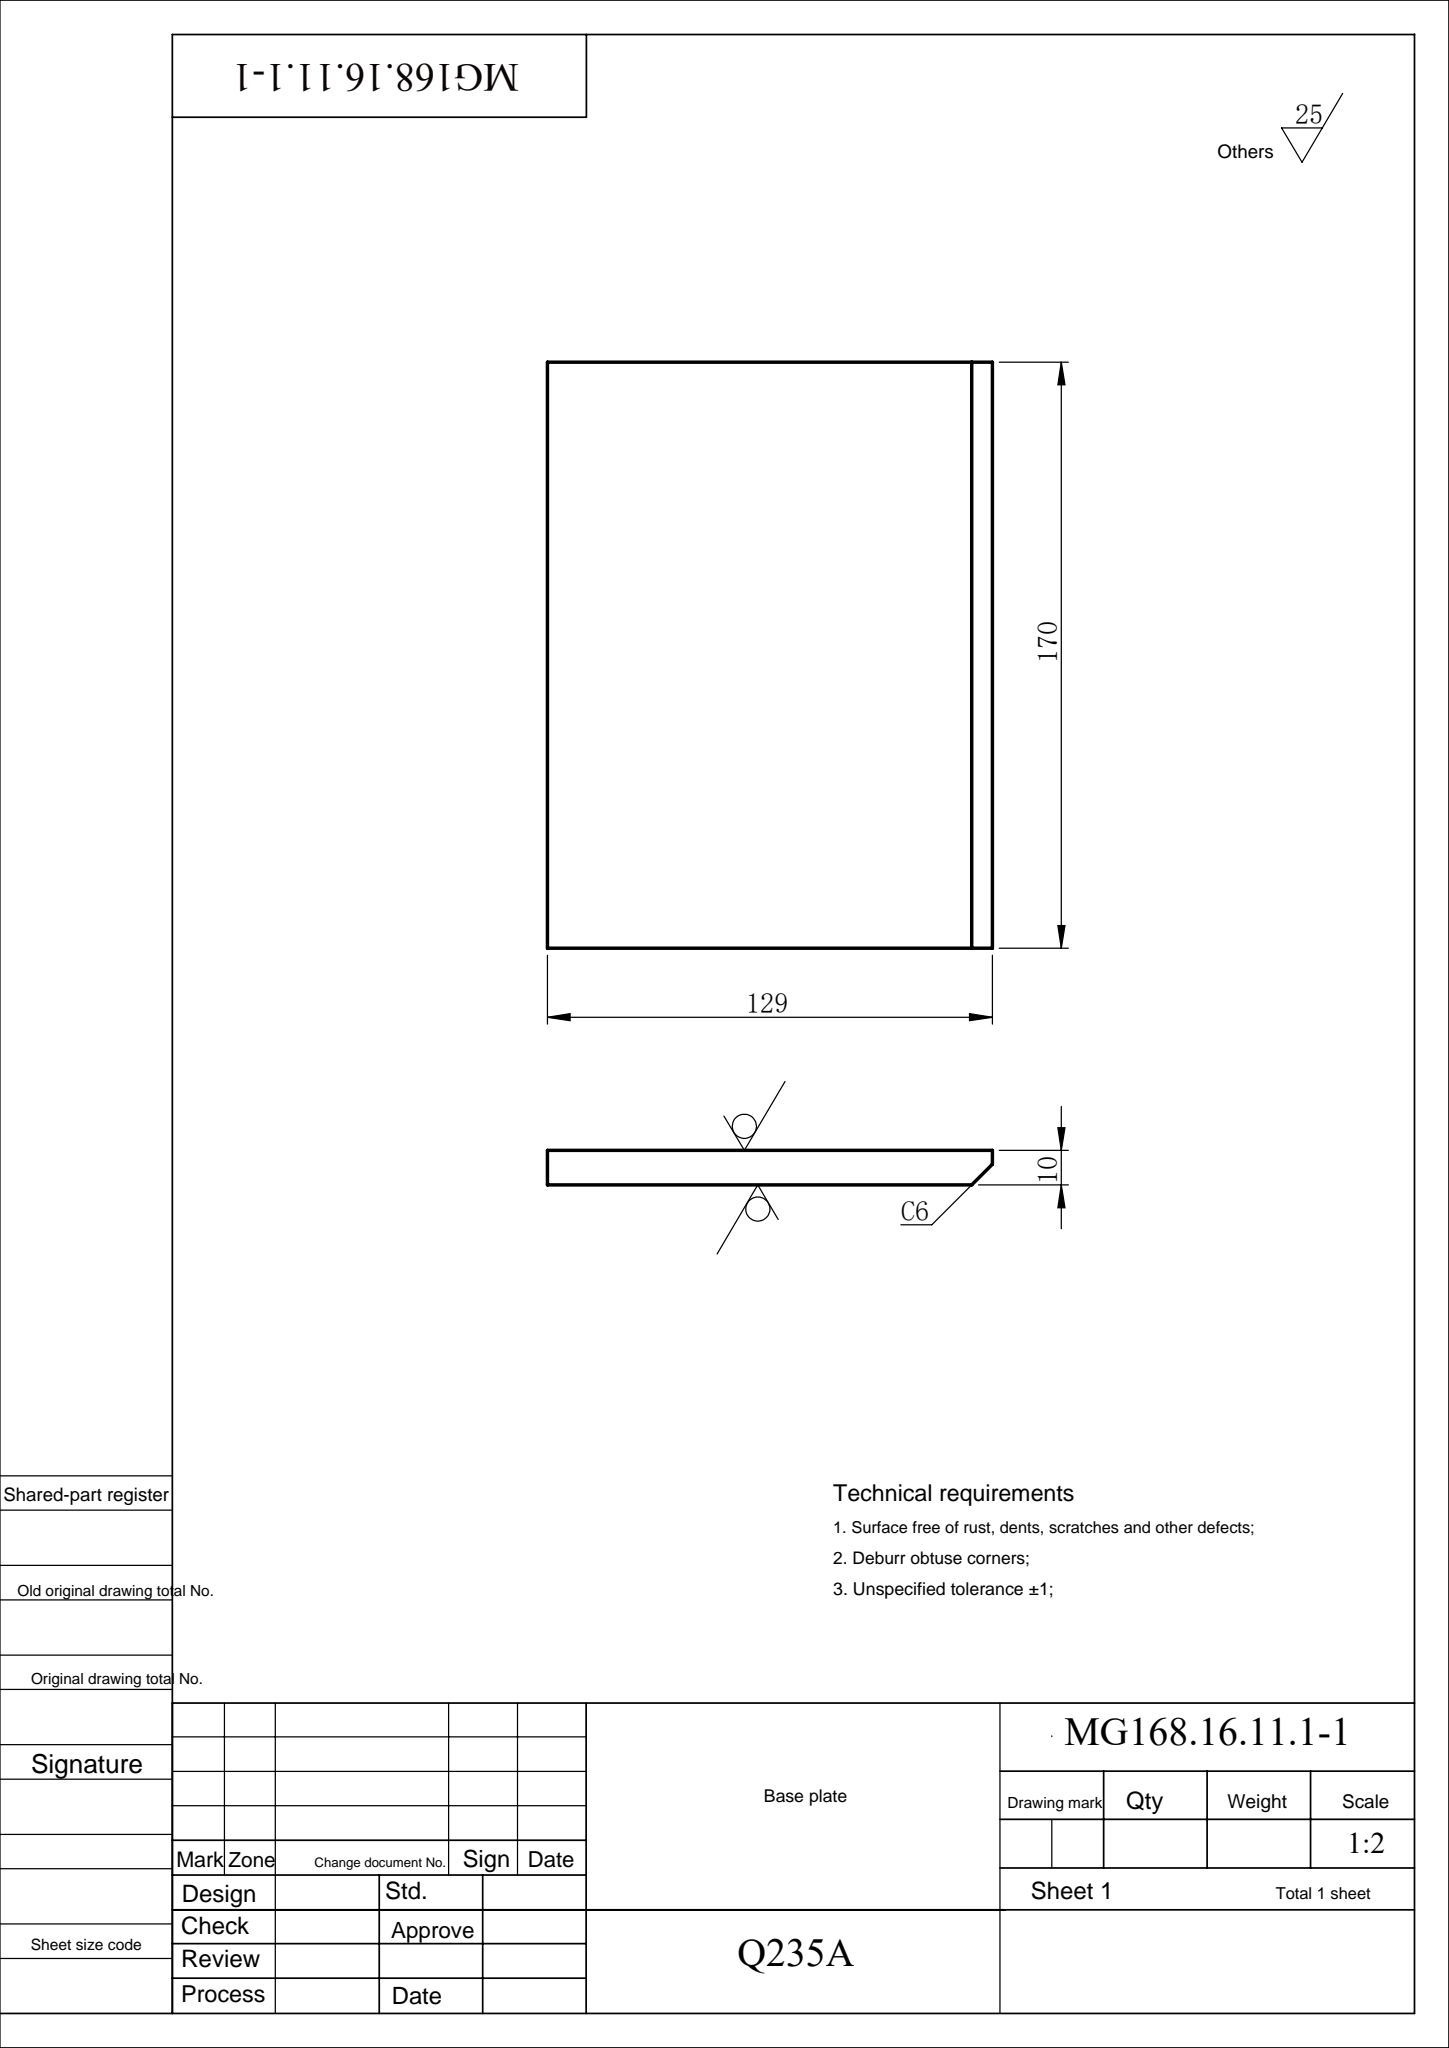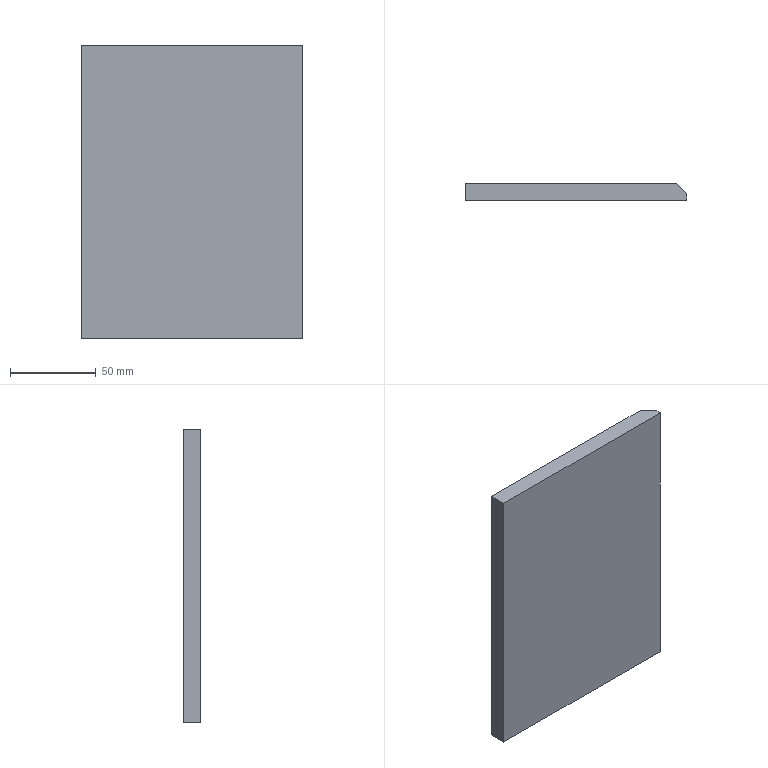Part | SolidWorks | features Chamfer 1, Extrusion 1 | 1 solid | 7 faces | box 129 x 10 x 170 mm | volume 216240 mm3 | plane 7
STEP:
#1=CARTESIAN_POINT('',(-58.,-5.,-85.));
#2=VERTEX_POINT('',#1);
#3=CARTESIAN_POINT('',(-58.,-5.,85.));
#4=VERTEX_POINT('',#3);
#5=CARTESIAN_POINT('',(-58.,-5.,-85.));
#6=DIRECTION('',(0.,0.,1.));
#7=VECTOR('',#6,1000.);
#8=LINE('',#5,#7);
#9=EDGE_CURVE('',#2,#4,#8,.T.);
#10=ORIENTED_EDGE('',*,*,#9,.T.);
#11=CARTESIAN_POINT('',(-58.,5.,85.));
#12=VERTEX_POINT('',#11);
#13=CARTESIAN_POINT('',(-58.,5.,85.));
#14=DIRECTION('',(0.,-1.,0.));
#15=VECTOR('',#14,1000.);
#16=LINE('',#13,#15);
#17=EDGE_CURVE('',#12,#4,#16,.T.);
#18=ORIENTED_EDGE('',*,*,#17,.F.);
#19=CARTESIAN_POINT('',(-58.,5.,-85.));
#20=VERTEX_POINT('',#19);
#21=CARTESIAN_POINT('',(-58.,5.,-85.));
#22=DIRECTION('',(0.,0.,1.));
#23=VECTOR('',#22,1000.);
#24=LINE('',#21,#23);
#25=EDGE_CURVE('',#20,#12,#24,.T.);
#26=ORIENTED_EDGE('',*,*,#25,.F.);
#27=CARTESIAN_POINT('',(-58.,5.,-85.));
#28=DIRECTION('',(0.,-1.,0.));
#29=VECTOR('',#28,1000.);
#30=LINE('',#27,#29);
#31=EDGE_CURVE('',#20,#2,#30,.T.);
#32=ORIENTED_EDGE('',*,*,#31,.T.);
#33=EDGE_LOOP('',(#10,#18,#26,#32));
#34=FACE_OUTER_BOUND('',#33,.T.);
#35=CARTESIAN_POINT('',(-58.,5.,-85.));
#36=DIRECTION('',(1.,0.,0.));
#37=DIRECTION('',(0.,0.,-1.));
#38=AXIS2_PLACEMENT_3D('',#35,#36,#37);
#39=PLANE('',#38);
#40=ADVANCED_FACE('',(#34),#39,.F.);
#41=CARTESIAN_POINT('',(71.,-1.,85.));
#42=VERTEX_POINT('',#41);
#43=CARTESIAN_POINT('',(71.,-5.,85.));
#44=VERTEX_POINT('',#43);
#45=CARTESIAN_POINT('',(71.,5.,85.));
#46=DIRECTION('',(0.,-1.,0.));
#47=VECTOR('',#46,1000.);
#48=LINE('',#45,#47);
#49=EDGE_CURVE('',#42,#44,#48,.T.);
#50=ORIENTED_EDGE('',*,*,#49,.F.);
#51=CARTESIAN_POINT('',(65.,5.,85.));
#52=VERTEX_POINT('',#51);
#53=CARTESIAN_POINT('',(65.,5.,85.));
#54=DIRECTION('',(-0.7071,0.7071,0.));
#55=VECTOR('',#54,1000.);
#56=LINE('',#53,#55);
#57=EDGE_CURVE('',#42,#52,#56,.T.);
#58=ORIENTED_EDGE('',*,*,#57,.T.);
#59=CARTESIAN_POINT('',(-58.,5.,85.));
#60=DIRECTION('',(1.,0.,0.));
#61=VECTOR('',#60,1000.);
#62=LINE('',#59,#61);
#63=EDGE_CURVE('',#12,#52,#62,.T.);
#64=ORIENTED_EDGE('',*,*,#63,.F.);
#65=ORIENTED_EDGE('',*,*,#17,.T.);
#66=CARTESIAN_POINT('',(-58.,-5.,85.));
#67=DIRECTION('',(1.,0.,0.));
#68=VECTOR('',#67,1000.);
#69=LINE('',#66,#68);
#70=EDGE_CURVE('',#4,#44,#69,.T.);
#71=ORIENTED_EDGE('',*,*,#70,.T.);
#72=EDGE_LOOP('',(#50,#58,#64,#65,#71));
#73=FACE_OUTER_BOUND('',#72,.T.);
#74=CARTESIAN_POINT('',(-58.,5.,85.));
#75=DIRECTION('',(0.,0.,-1.));
#76=DIRECTION('',(-1.,0.,0.));
#77=AXIS2_PLACEMENT_3D('',#74,#75,#76);
#78=PLANE('',#77);
#79=ADVANCED_FACE('',(#73),#78,.F.);
#80=CARTESIAN_POINT('',(71.,-1.,-85.));
#81=VERTEX_POINT('',#80);
#82=CARTESIAN_POINT('',(71.,-5.,-85.));
#83=VERTEX_POINT('',#82);
#84=CARTESIAN_POINT('',(71.,5.,-85.));
#85=DIRECTION('',(0.,-1.,0.));
#86=VECTOR('',#85,1000.);
#87=LINE('',#84,#86);
#88=EDGE_CURVE('',#81,#83,#87,.T.);
#89=ORIENTED_EDGE('',*,*,#88,.F.);
#90=CARTESIAN_POINT('',(71.,-1.,85.));
#91=DIRECTION('',(0.,0.,1.));
#92=VECTOR('',#91,1000.);
#93=LINE('',#90,#92);
#94=EDGE_CURVE('',#81,#42,#93,.T.);
#95=ORIENTED_EDGE('',*,*,#94,.T.);
#96=ORIENTED_EDGE('',*,*,#49,.T.);
#97=CARTESIAN_POINT('',(71.,-5.,-85.));
#98=DIRECTION('',(0.,0.,-1.));
#99=VECTOR('',#98,1000.);
#100=LINE('',#97,#99);
#101=EDGE_CURVE('',#44,#83,#100,.T.);
#102=ORIENTED_EDGE('',*,*,#101,.T.);
#103=EDGE_LOOP('',(#89,#95,#96,#102));
#104=FACE_OUTER_BOUND('',#103,.T.);
#105=CARTESIAN_POINT('',(71.,5.,-85.));
#106=DIRECTION('',(-1.,0.,0.));
#107=DIRECTION('',(0.,0.,1.));
#108=AXIS2_PLACEMENT_3D('',#105,#106,#107);
#109=PLANE('',#108);
#110=ADVANCED_FACE('',(#104),#109,.F.);
#111=CARTESIAN_POINT('',(65.,5.,-85.));
#112=VERTEX_POINT('',#111);
#113=CARTESIAN_POINT('',(-58.,5.,-85.));
#114=DIRECTION('',(-1.,0.,0.));
#115=VECTOR('',#114,1000.);
#116=LINE('',#113,#115);
#117=EDGE_CURVE('',#112,#20,#116,.T.);
#118=ORIENTED_EDGE('',*,*,#117,.F.);
#119=CARTESIAN_POINT('',(65.,5.,-85.));
#120=DIRECTION('',(0.7071,-0.7071,0.));
#121=VECTOR('',#120,1000.);
#122=LINE('',#119,#121);
#123=EDGE_CURVE('',#112,#81,#122,.T.);
#124=ORIENTED_EDGE('',*,*,#123,.T.);
#125=ORIENTED_EDGE('',*,*,#88,.T.);
#126=CARTESIAN_POINT('',(-58.,-5.,-85.));
#127=DIRECTION('',(-1.,0.,0.));
#128=VECTOR('',#127,1000.);
#129=LINE('',#126,#128);
#130=EDGE_CURVE('',#83,#2,#129,.T.);
#131=ORIENTED_EDGE('',*,*,#130,.T.);
#132=ORIENTED_EDGE('',*,*,#31,.F.);
#133=EDGE_LOOP('',(#118,#124,#125,#131,#132));
#134=FACE_OUTER_BOUND('',#133,.T.);
#135=CARTESIAN_POINT('',(-58.,5.,-85.));
#136=DIRECTION('',(0.,0.,1.));
#137=DIRECTION('',(1.,0.,0.));
#138=AXIS2_PLACEMENT_3D('',#135,#136,#137);
#139=PLANE('',#138);
#140=ADVANCED_FACE('',(#134),#139,.F.);
#141=ORIENTED_EDGE('',*,*,#63,.T.);
#142=CARTESIAN_POINT('',(65.,5.,-85.));
#143=DIRECTION('',(0.,0.,-1.));
#144=VECTOR('',#143,1000.);
#145=LINE('',#142,#144);
#146=EDGE_CURVE('',#52,#112,#145,.T.);
#147=ORIENTED_EDGE('',*,*,#146,.T.);
#148=ORIENTED_EDGE('',*,*,#117,.T.);
#149=ORIENTED_EDGE('',*,*,#25,.T.);
#150=EDGE_LOOP('',(#141,#147,#148,#149));
#151=FACE_OUTER_BOUND('',#150,.T.);
#152=CARTESIAN_POINT('',(0.,5.,0.));
#153=DIRECTION('',(0.,1.,0.));
#154=DIRECTION('',(0.,0.,1.));
#155=AXIS2_PLACEMENT_3D('',#152,#153,#154);
#156=PLANE('',#155);
#157=ADVANCED_FACE('',(#151),#156,.T.);
#158=ORIENTED_EDGE('',*,*,#9,.F.);
#159=ORIENTED_EDGE('',*,*,#130,.F.);
#160=ORIENTED_EDGE('',*,*,#101,.F.);
#161=ORIENTED_EDGE('',*,*,#70,.F.);
#162=EDGE_LOOP('',(#158,#159,#160,#161));
#163=FACE_OUTER_BOUND('',#162,.T.);
#164=CARTESIAN_POINT('',(0.,-5.,0.));
#165=DIRECTION('',(0.,1.,0.));
#166=DIRECTION('',(0.,0.,1.));
#167=AXIS2_PLACEMENT_3D('',#164,#165,#166);
#168=PLANE('',#167);
#169=ADVANCED_FACE('',(#163),#168,.F.);
#170=ORIENTED_EDGE('',*,*,#57,.F.);
#171=ORIENTED_EDGE('',*,*,#94,.F.);
#172=ORIENTED_EDGE('',*,*,#123,.F.);
#173=ORIENTED_EDGE('',*,*,#146,.F.);
#174=EDGE_LOOP('',(#170,#171,#172,#173));
#175=FACE_OUTER_BOUND('',#174,.T.);
#176=CARTESIAN_POINT('',(65.,5.,0.));
#177=DIRECTION('',(0.7071,0.7071,0.));
#178=DIRECTION('',(0.,0.,1.));
#179=AXIS2_PLACEMENT_3D('',#176,#177,#178);
#180=PLANE('',#179);
#181=ADVANCED_FACE('',(#175),#180,.T.);
#182=CLOSED_SHELL('',(#40,#79,#110,#140,#157,#169,#181));
#183=MANIFOLD_SOLID_BREP('',#182);
#184=CARTESIAN_POINT('',(0.,0.,0.));
#185=DIRECTION('',(0.,0.,1.));
#186=DIRECTION('',(1.,0.,0.));
#187=AXIS2_PLACEMENT_3D('',#184,#185,#186);
#188=(LENGTH_UNIT()NAMED_UNIT(*)SI_UNIT(.MILLI.,.METRE.));
#189=UNCERTAINTY_MEASURE_WITH_UNIT(LENGTH_MEASURE(0.00001),#188,'','');
#190=(NAMED_UNIT(*)PLANE_ANGLE_UNIT()SI_UNIT($,.RADIAN.));
#191=(NAMED_UNIT(*)SI_UNIT($,.STERADIAN.)SOLID_ANGLE_UNIT());
#192=(GEOMETRIC_REPRESENTATION_CONTEXT(3)GLOBAL_UNCERTAINTY_ASSIGNED_CONTEXT((#189))GLOBAL_UNIT_ASSIGNED_CONTEXT((#188,#190,#191))REPRESENTATION_CONTEXT('',''));
#193=ADVANCED_BREP_SHAPE_REPRESENTATION('',(#183,#187),#192);